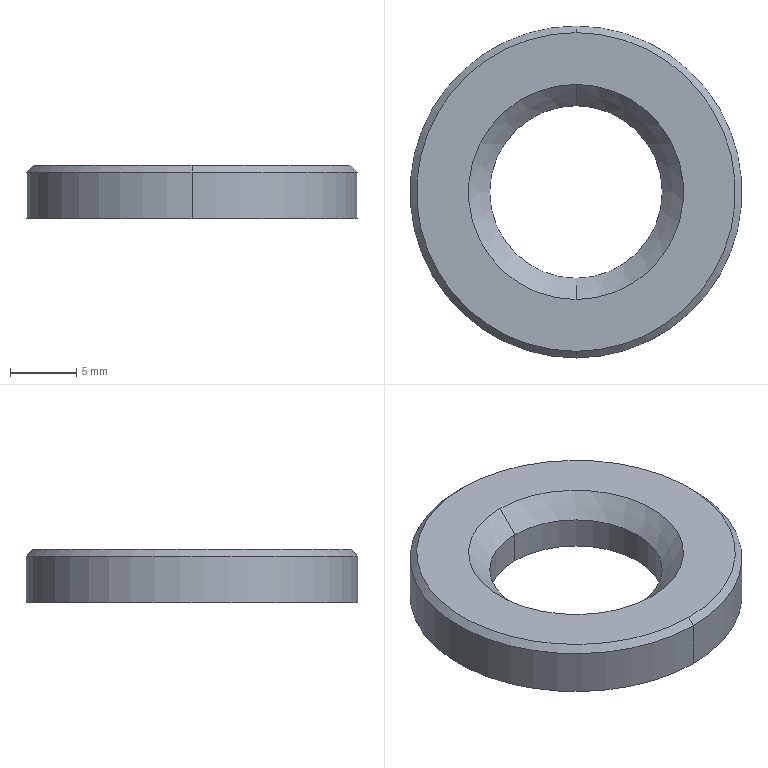Part | STEP file | Microwave Drying Flat Conveyor-rondelle_iso_7416-12 | 1 solid | 10 faces | box 25 x 25 x 4 mm | volume 1366 mm3 | cone 4 | cylinder 4 | plane 2 | commonest cylinder face diameters 13 x2 25 x2
STEP:
#1=CARTESIAN_POINT('',(0.,-6.5,2.4));
#2=VERTEX_POINT('',#1);
#3=CARTESIAN_POINT('',(0.,6.5,2.4));
#4=VERTEX_POINT('',#3);
#5=CARTESIAN_POINT('',(0.,0.,2.4));
#6=DIRECTION('',(0.,0.,-1.));
#7=DIRECTION('',(0.,1.,0.));
#8=AXIS2_PLACEMENT_3D('',#5,#6,#7);
#9=CIRCLE('',#8,6.5);
#10=EDGE_CURVE('',#2,#4,#9,.T.);
#11=ORIENTED_EDGE('',*,*,#10,.T.);
#12=CARTESIAN_POINT('',(0.,8.1,4.));
#13=VERTEX_POINT('',#12);
#14=CARTESIAN_POINT('',(0.,8.1,4.));
#15=DIRECTION('',(0.,0.7071,0.7071));
#16=VECTOR('',#15,1000.);
#17=LINE('',#14,#16);
#18=EDGE_CURVE('',#4,#13,#17,.T.);
#19=ORIENTED_EDGE('',*,*,#18,.T.);
#20=CARTESIAN_POINT('',(0.,-8.1,4.));
#21=VERTEX_POINT('',#20);
#22=CARTESIAN_POINT('',(0.,0.,4.));
#23=DIRECTION('',(0.,0.,-1.));
#24=DIRECTION('',(0.,1.,0.));
#25=AXIS2_PLACEMENT_3D('',#22,#23,#24);
#26=CIRCLE('',#25,8.1);
#27=EDGE_CURVE('',#21,#13,#26,.T.);
#28=ORIENTED_EDGE('',*,*,#27,.F.);
#29=CARTESIAN_POINT('',(0.,-8.1,4.));
#30=DIRECTION('',(0.,-0.7071,0.7071));
#31=VECTOR('',#30,1000.);
#32=LINE('',#29,#31);
#33=EDGE_CURVE('',#2,#21,#32,.T.);
#34=ORIENTED_EDGE('',*,*,#33,.F.);
#35=EDGE_LOOP('',(#11,#19,#28,#34));
#36=FACE_OUTER_BOUND('',#35,.T.);
#37=CARTESIAN_POINT('',(0.,0.,4.));
#38=DIRECTION('',(0.,0.,1.));
#39=DIRECTION('',(0.,-1.,0.));
#40=AXIS2_PLACEMENT_3D('',#37,#38,#39);
#41=CONICAL_SURFACE('',#40,8.1,0.7854);
#42=ADVANCED_FACE('',(#36),#41,.F.);
#43=CARTESIAN_POINT('',(0.,12.,4.));
#44=VERTEX_POINT('',#43);
#45=CARTESIAN_POINT('',(0.,-12.,4.));
#46=VERTEX_POINT('',#45);
#47=CARTESIAN_POINT('',(0.,0.,4.));
#48=DIRECTION('',(0.,0.,-1.));
#49=DIRECTION('',(0.,1.,0.));
#50=AXIS2_PLACEMENT_3D('',#47,#48,#49);
#51=CIRCLE('',#50,12.);
#52=EDGE_CURVE('',#44,#46,#51,.T.);
#53=ORIENTED_EDGE('',*,*,#52,.T.);
#54=CARTESIAN_POINT('',(0.,-12.5,3.5));
#55=VERTEX_POINT('',#54);
#56=CARTESIAN_POINT('',(0.,-12.5,3.5));
#57=DIRECTION('',(0.,-0.7071,-0.7071));
#58=VECTOR('',#57,1000.);
#59=LINE('',#56,#58);
#60=EDGE_CURVE('',#46,#55,#59,.T.);
#61=ORIENTED_EDGE('',*,*,#60,.T.);
#62=CARTESIAN_POINT('',(0.,12.5,3.5));
#63=VERTEX_POINT('',#62);
#64=CARTESIAN_POINT('',(0.,0.,3.5));
#65=DIRECTION('',(0.,0.,-1.));
#66=DIRECTION('',(0.,1.,0.));
#67=AXIS2_PLACEMENT_3D('',#64,#65,#66);
#68=CIRCLE('',#67,12.5);
#69=EDGE_CURVE('',#63,#55,#68,.T.);
#70=ORIENTED_EDGE('',*,*,#69,.F.);
#71=CARTESIAN_POINT('',(0.,12.5,3.5));
#72=DIRECTION('',(0.,0.7071,-0.7071));
#73=VECTOR('',#72,1000.);
#74=LINE('',#71,#73);
#75=EDGE_CURVE('',#44,#63,#74,.T.);
#76=ORIENTED_EDGE('',*,*,#75,.F.);
#77=EDGE_LOOP('',(#53,#61,#70,#76));
#78=FACE_OUTER_BOUND('',#77,.T.);
#79=CARTESIAN_POINT('',(0.,0.,3.5));
#80=DIRECTION('',(0.,0.,-1.));
#81=DIRECTION('',(0.,1.,0.));
#82=AXIS2_PLACEMENT_3D('',#79,#80,#81);
#83=CONICAL_SURFACE('',#82,12.5,0.7854);
#84=ADVANCED_FACE('',(#78),#83,.T.);
#85=ORIENTED_EDGE('',*,*,#69,.T.);
#86=CARTESIAN_POINT('',(0.,-12.5,0.));
#87=VERTEX_POINT('',#86);
#88=CARTESIAN_POINT('',(0.,-12.5,0.));
#89=DIRECTION('',(0.,0.,-1.));
#90=VECTOR('',#89,1000.);
#91=LINE('',#88,#90);
#92=EDGE_CURVE('',#55,#87,#91,.T.);
#93=ORIENTED_EDGE('',*,*,#92,.T.);
#94=CARTESIAN_POINT('',(0.,12.5,0.));
#95=VERTEX_POINT('',#94);
#96=CARTESIAN_POINT('',(0.,0.,0.));
#97=DIRECTION('',(0.,0.,-1.));
#98=DIRECTION('',(0.,1.,0.));
#99=AXIS2_PLACEMENT_3D('',#96,#97,#98);
#100=CIRCLE('',#99,12.5);
#101=EDGE_CURVE('',#95,#87,#100,.T.);
#102=ORIENTED_EDGE('',*,*,#101,.F.);
#103=CARTESIAN_POINT('',(0.,12.5,0.));
#104=DIRECTION('',(0.,0.,-1.));
#105=VECTOR('',#104,1000.);
#106=LINE('',#103,#105);
#107=EDGE_CURVE('',#63,#95,#106,.T.);
#108=ORIENTED_EDGE('',*,*,#107,.F.);
#109=EDGE_LOOP('',(#85,#93,#102,#108));
#110=FACE_OUTER_BOUND('',#109,.T.);
#111=CARTESIAN_POINT('',(0.,0.,0.));
#112=DIRECTION('',(0.,0.,-1.));
#113=DIRECTION('',(0.,1.,0.));
#114=AXIS2_PLACEMENT_3D('',#111,#112,#113);
#115=CYLINDRICAL_SURFACE('',#114,12.5);
#116=ADVANCED_FACE('',(#110),#115,.T.);
#117=ORIENTED_EDGE('',*,*,#10,.F.);
#118=CARTESIAN_POINT('',(0.,-6.5,0.));
#119=VERTEX_POINT('',#118);
#120=CARTESIAN_POINT('',(0.,-6.5,0.));
#121=DIRECTION('',(0.,0.,-1.));
#122=VECTOR('',#121,1000.);
#123=LINE('',#120,#122);
#124=EDGE_CURVE('',#2,#119,#123,.T.);
#125=ORIENTED_EDGE('',*,*,#124,.T.);
#126=CARTESIAN_POINT('',(0.,6.5,0.));
#127=VERTEX_POINT('',#126);
#128=CARTESIAN_POINT('',(0.,0.,0.));
#129=DIRECTION('',(0.,0.,-1.));
#130=DIRECTION('',(0.,1.,0.));
#131=AXIS2_PLACEMENT_3D('',#128,#129,#130);
#132=CIRCLE('',#131,6.5);
#133=EDGE_CURVE('',#119,#127,#132,.T.);
#134=ORIENTED_EDGE('',*,*,#133,.T.);
#135=CARTESIAN_POINT('',(0.,6.5,0.));
#136=DIRECTION('',(0.,0.,-1.));
#137=VECTOR('',#136,1000.);
#138=LINE('',#135,#137);
#139=EDGE_CURVE('',#4,#127,#138,.T.);
#140=ORIENTED_EDGE('',*,*,#139,.F.);
#141=EDGE_LOOP('',(#117,#125,#134,#140));
#142=FACE_OUTER_BOUND('',#141,.T.);
#143=CARTESIAN_POINT('',(0.,0.,0.));
#144=DIRECTION('',(0.,0.,-1.));
#145=DIRECTION('',(0.,1.,0.));
#146=AXIS2_PLACEMENT_3D('',#143,#144,#145);
#147=CYLINDRICAL_SURFACE('',#146,6.5);
#148=ADVANCED_FACE('',(#142),#147,.F.);
#149=ORIENTED_EDGE('',*,*,#124,.F.);
#150=CARTESIAN_POINT('',(0.,0.,2.4));
#151=DIRECTION('',(0.,0.,-1.));
#152=DIRECTION('',(0.,1.,0.));
#153=AXIS2_PLACEMENT_3D('',#150,#151,#152);
#154=CIRCLE('',#153,6.5);
#155=EDGE_CURVE('',#4,#2,#154,.T.);
#156=ORIENTED_EDGE('',*,*,#155,.F.);
#157=ORIENTED_EDGE('',*,*,#139,.T.);
#158=CARTESIAN_POINT('',(0.,0.,0.));
#159=DIRECTION('',(0.,0.,-1.));
#160=DIRECTION('',(0.,1.,0.));
#161=AXIS2_PLACEMENT_3D('',#158,#159,#160);
#162=CIRCLE('',#161,6.5);
#163=EDGE_CURVE('',#127,#119,#162,.T.);
#164=ORIENTED_EDGE('',*,*,#163,.T.);
#165=EDGE_LOOP('',(#149,#156,#157,#164));
#166=FACE_OUTER_BOUND('',#165,.T.);
#167=CARTESIAN_POINT('',(0.,0.,0.));
#168=DIRECTION('',(0.,0.,-1.));
#169=DIRECTION('',(0.,1.,0.));
#170=AXIS2_PLACEMENT_3D('',#167,#168,#169);
#171=CYLINDRICAL_SURFACE('',#170,6.5);
#172=ADVANCED_FACE('',(#166),#171,.F.);
#173=ORIENTED_EDGE('',*,*,#101,.T.);
#174=CARTESIAN_POINT('',(0.,0.,0.));
#175=DIRECTION('',(0.,0.,-1.));
#176=DIRECTION('',(0.,1.,0.));
#177=AXIS2_PLACEMENT_3D('',#174,#175,#176);
#178=CIRCLE('',#177,12.5);
#179=EDGE_CURVE('',#87,#95,#178,.T.);
#180=ORIENTED_EDGE('',*,*,#179,.T.);
#181=EDGE_LOOP('',(#173,#180));
#182=FACE_OUTER_BOUND('',#181,.T.);
#183=ORIENTED_EDGE('',*,*,#163,.F.);
#184=ORIENTED_EDGE('',*,*,#133,.F.);
#185=EDGE_LOOP('',(#183,#184));
#186=FACE_BOUND('',#185,.T.);
#187=CARTESIAN_POINT('',(6.5,0.,0.));
#188=DIRECTION('',(0.,0.,-1.));
#189=DIRECTION('',(0.,1.,0.));
#190=AXIS2_PLACEMENT_3D('',#187,#188,#189);
#191=PLANE('',#190);
#192=ADVANCED_FACE('',(#182,#186),#191,.T.);
#193=ORIENTED_EDGE('',*,*,#92,.F.);
#194=CARTESIAN_POINT('',(0.,0.,3.5));
#195=DIRECTION('',(0.,0.,-1.));
#196=DIRECTION('',(0.,1.,0.));
#197=AXIS2_PLACEMENT_3D('',#194,#195,#196);
#198=CIRCLE('',#197,12.5);
#199=EDGE_CURVE('',#55,#63,#198,.T.);
#200=ORIENTED_EDGE('',*,*,#199,.T.);
#201=ORIENTED_EDGE('',*,*,#107,.T.);
#202=ORIENTED_EDGE('',*,*,#179,.F.);
#203=EDGE_LOOP('',(#193,#200,#201,#202));
#204=FACE_OUTER_BOUND('',#203,.T.);
#205=CARTESIAN_POINT('',(0.,0.,0.));
#206=DIRECTION('',(0.,0.,-1.));
#207=DIRECTION('',(0.,1.,0.));
#208=AXIS2_PLACEMENT_3D('',#205,#206,#207);
#209=CYLINDRICAL_SURFACE('',#208,12.5);
#210=ADVANCED_FACE('',(#204),#209,.T.);
#211=ORIENTED_EDGE('',*,*,#60,.F.);
#212=CARTESIAN_POINT('',(0.,0.,4.));
#213=DIRECTION('',(0.,0.,-1.));
#214=DIRECTION('',(0.,1.,0.));
#215=AXIS2_PLACEMENT_3D('',#212,#213,#214);
#216=CIRCLE('',#215,12.);
#217=EDGE_CURVE('',#46,#44,#216,.T.);
#218=ORIENTED_EDGE('',*,*,#217,.T.);
#219=ORIENTED_EDGE('',*,*,#75,.T.);
#220=ORIENTED_EDGE('',*,*,#199,.F.);
#221=EDGE_LOOP('',(#211,#218,#219,#220));
#222=FACE_OUTER_BOUND('',#221,.T.);
#223=CARTESIAN_POINT('',(0.,0.,3.5));
#224=DIRECTION('',(0.,0.,-1.));
#225=DIRECTION('',(0.,1.,0.));
#226=AXIS2_PLACEMENT_3D('',#223,#224,#225);
#227=CONICAL_SURFACE('',#226,12.5,0.7854);
#228=ADVANCED_FACE('',(#222),#227,.T.);
#229=ORIENTED_EDGE('',*,*,#27,.T.);
#230=CARTESIAN_POINT('',(0.,0.,4.));
#231=DIRECTION('',(0.,0.,-1.));
#232=DIRECTION('',(0.,1.,0.));
#233=AXIS2_PLACEMENT_3D('',#230,#231,#232);
#234=CIRCLE('',#233,8.1);
#235=EDGE_CURVE('',#13,#21,#234,.T.);
#236=ORIENTED_EDGE('',*,*,#235,.T.);
#237=EDGE_LOOP('',(#229,#236));
#238=FACE_BOUND('',#237,.T.);
#239=ORIENTED_EDGE('',*,*,#52,.F.);
#240=ORIENTED_EDGE('',*,*,#217,.F.);
#241=EDGE_LOOP('',(#239,#240));
#242=FACE_OUTER_BOUND('',#241,.T.);
#243=CARTESIAN_POINT('',(12.,0.,4.));
#244=DIRECTION('',(0.,0.,1.));
#245=DIRECTION('',(0.,-1.,0.));
#246=AXIS2_PLACEMENT_3D('',#243,#244,#245);
#247=PLANE('',#246);
#248=ADVANCED_FACE('',(#238,#242),#247,.T.);
#249=ORIENTED_EDGE('',*,*,#18,.F.);
#250=ORIENTED_EDGE('',*,*,#155,.T.);
#251=ORIENTED_EDGE('',*,*,#33,.T.);
#252=ORIENTED_EDGE('',*,*,#235,.F.);
#253=EDGE_LOOP('',(#249,#250,#251,#252));
#254=FACE_OUTER_BOUND('',#253,.T.);
#255=CARTESIAN_POINT('',(0.,0.,4.));
#256=DIRECTION('',(0.,0.,1.));
#257=DIRECTION('',(0.,-1.,0.));
#258=AXIS2_PLACEMENT_3D('',#255,#256,#257);
#259=CONICAL_SURFACE('',#258,8.1,0.7854);
#260=ADVANCED_FACE('',(#254),#259,.F.);
#261=CLOSED_SHELL('',(#42,#84,#116,#148,#172,#192,#210,#228,#248,#260));
#262=MANIFOLD_SOLID_BREP('',#261);
#263=CARTESIAN_POINT('',(0.,0.,0.));
#264=DIRECTION('',(0.,0.,1.));
#265=DIRECTION('',(1.,0.,0.));
#266=AXIS2_PLACEMENT_3D('',#263,#264,#265);
#267=(LENGTH_UNIT()NAMED_UNIT(*)SI_UNIT(.MILLI.,.METRE.));
#268=UNCERTAINTY_MEASURE_WITH_UNIT(LENGTH_MEASURE(0.00001),#267,'','');
#269=(NAMED_UNIT(*)PLANE_ANGLE_UNIT()SI_UNIT($,.RADIAN.));
#270=(NAMED_UNIT(*)SI_UNIT($,.STERADIAN.)SOLID_ANGLE_UNIT());
#271=(GEOMETRIC_REPRESENTATION_CONTEXT(3)GLOBAL_UNCERTAINTY_ASSIGNED_CONTEXT((#268))GLOBAL_UNIT_ASSIGNED_CONTEXT((#267,#269,#270))REPRESENTATION_CONTEXT('',''));
#272=ADVANCED_BREP_SHAPE_REPRESENTATION('',(#262,#266),#271);